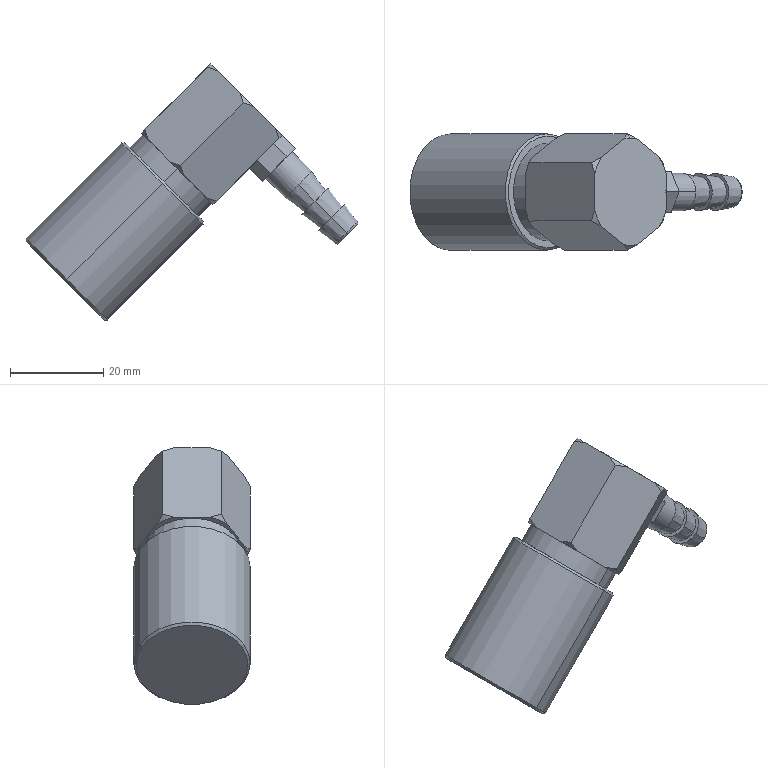Part | STEP file | 4-20.sldasm-Part-54 | 1 solid | 52 faces | box 71.345 x 25 x 55.031 mm | volume 25800 mm3 | cone 24 | plane 20 | cylinder 6 | torus 2 | commonest cylinder face diameters 8 x2 21 x2 25 x2